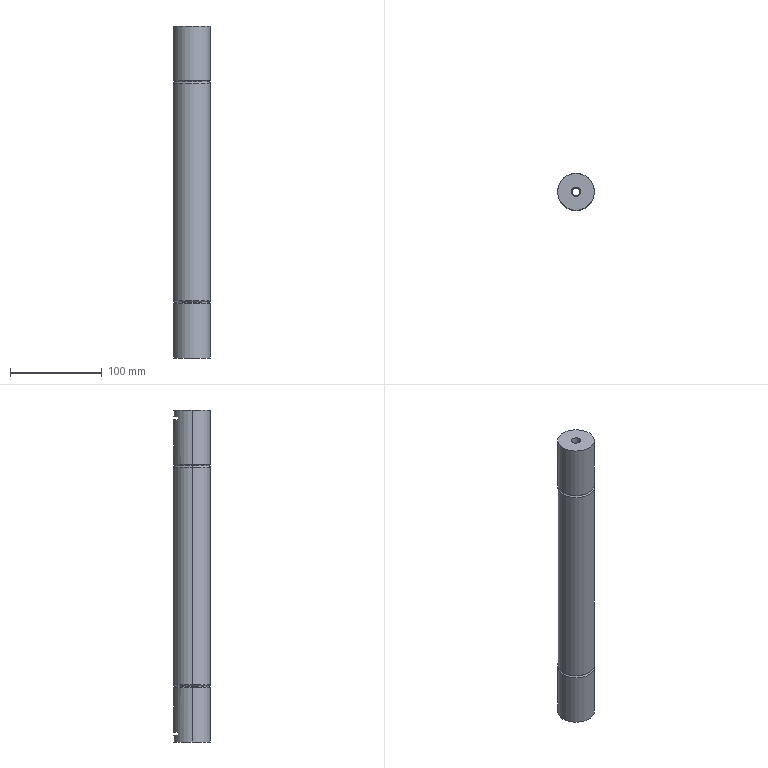Part | STEP file | LM-05-1231 | 1 solid | 38 faces | box 40 x 40 x 361 mm | volume 430990 mm3 | torus 12 | cylinder 12 | plane 10 | cone 4 | commonest cylinder face diameters 40 x6 3 x4 8.5 x2